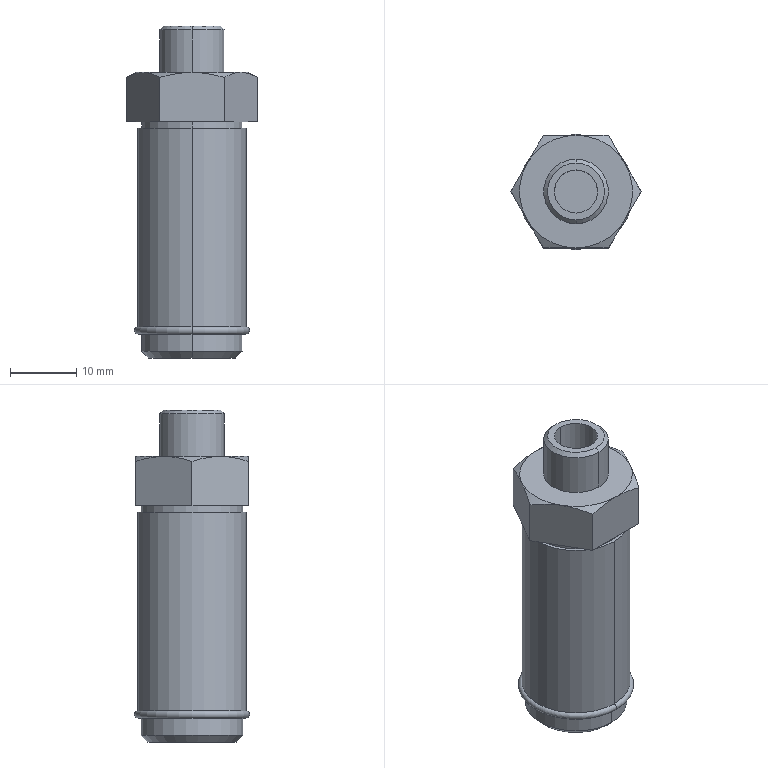Part | SolidWorks | features RefAxis 3, 3DProfileFeature 1, ICE 1, Revolution 1 | 1 solid | 40 faces | box 19.63 x 17.35 x 50 mm | volume 8637 mm3 | plane 14 | cylinder 12 | cone 12 | torus 2 | commonest cylinder face diameters 15.3 x4 6.485 x2 8.566 x2 9.728 x2 16.3 x2
STEP:
#1=CARTESIAN_POINT('',(0.,-4.864,39.4));
#2=VERTEX_POINT('',#1);
#3=CARTESIAN_POINT('',(0.,4.864,39.4));
#4=VERTEX_POINT('',#3);
#5=CARTESIAN_POINT('',(0.,0.,39.4));
#6=DIRECTION('',(0.,0.,1.));
#7=DIRECTION('',(0.,-1.,0.));
#8=AXIS2_PLACEMENT_3D('',#5,#6,#7);
#9=CIRCLE('',#8,4.864);
#10=EDGE_CURVE('',#2,#4,#9,.T.);
#11=ORIENTED_EDGE('',*,*,#10,.T.);
#12=CARTESIAN_POINT('',(0.,4.864,45.819));
#13=VERTEX_POINT('',#12);
#14=CARTESIAN_POINT('',(0.,4.864,-3.6));
#15=DIRECTION('',(0.,0.,1.));
#16=VECTOR('',#15,1000.);
#17=LINE('',#14,#16);
#18=EDGE_CURVE('',#4,#13,#17,.T.);
#19=ORIENTED_EDGE('',*,*,#18,.T.);
#20=CARTESIAN_POINT('',(0.,-4.864,45.819));
#21=VERTEX_POINT('',#20);
#22=CARTESIAN_POINT('',(0.,0.,45.819));
#23=DIRECTION('',(0.,0.,1.));
#24=DIRECTION('',(0.,-1.,0.));
#25=AXIS2_PLACEMENT_3D('',#22,#23,#24);
#26=CIRCLE('',#25,4.864);
#27=EDGE_CURVE('',#21,#13,#26,.T.);
#28=ORIENTED_EDGE('',*,*,#27,.F.);
#29=CARTESIAN_POINT('',(0.,-4.864,-3.6));
#30=DIRECTION('',(0.,0.,1.));
#31=VECTOR('',#30,1000.);
#32=LINE('',#29,#31);
#33=EDGE_CURVE('',#2,#21,#32,.T.);
#34=ORIENTED_EDGE('',*,*,#33,.F.);
#35=EDGE_LOOP('',(#11,#19,#28,#34));
#36=FACE_OUTER_BOUND('',#35,.T.);
#37=CARTESIAN_POINT('',(0.,0.,-3.6));
#38=DIRECTION('',(0.,0.,1.));
#39=DIRECTION('',(0.,-1.,0.));
#40=AXIS2_PLACEMENT_3D('',#37,#38,#39);
#41=CYLINDRICAL_SURFACE('',#40,4.864);
#42=ADVANCED_FACE('',(#36),#41,.T.);
#43=CARTESIAN_POINT('',(0.,-4.283,46.4));
#44=VERTEX_POINT('',#43);
#45=CARTESIAN_POINT('',(0.,4.283,46.4));
#46=VERTEX_POINT('',#45);
#47=CARTESIAN_POINT('',(0.,0.,46.4));
#48=DIRECTION('',(0.,0.,1.));
#49=DIRECTION('',(0.,-1.,0.));
#50=AXIS2_PLACEMENT_3D('',#47,#48,#49);
#51=CIRCLE('',#50,4.283);
#52=EDGE_CURVE('',#44,#46,#51,.T.);
#53=ORIENTED_EDGE('',*,*,#52,.F.);
#54=CARTESIAN_POINT('',(0.,-4.864,45.819));
#55=DIRECTION('',(0.,-0.7071,-0.7071));
#56=VECTOR('',#55,1000.);
#57=LINE('',#54,#56);
#58=EDGE_CURVE('',#44,#21,#57,.T.);
#59=ORIENTED_EDGE('',*,*,#58,.T.);
#60=ORIENTED_EDGE('',*,*,#27,.T.);
#61=CARTESIAN_POINT('',(0.,4.864,45.819));
#62=DIRECTION('',(0.,0.7071,-0.7071));
#63=VECTOR('',#62,1000.);
#64=LINE('',#61,#63);
#65=EDGE_CURVE('',#46,#13,#64,.T.);
#66=ORIENTED_EDGE('',*,*,#65,.F.);
#67=EDGE_LOOP('',(#53,#59,#60,#66));
#68=FACE_OUTER_BOUND('',#67,.T.);
#69=CARTESIAN_POINT('',(0.,0.,45.819));
#70=DIRECTION('',(0.,0.,-1.));
#71=DIRECTION('',(0.,1.,0.));
#72=AXIS2_PLACEMENT_3D('',#69,#70,#71);
#73=CONICAL_SURFACE('',#72,4.864,0.7854);
#74=ADVANCED_FACE('',(#68),#73,.T.);
#75=CARTESIAN_POINT('',(0.,3.243,26.4));
#76=VERTEX_POINT('',#75);
#77=CARTESIAN_POINT('',(0.,-3.243,26.4));
#78=VERTEX_POINT('',#77);
#79=CARTESIAN_POINT('',(0.,0.,26.4));
#80=DIRECTION('',(0.,0.,1.));
#81=DIRECTION('',(0.,-1.,0.));
#82=AXIS2_PLACEMENT_3D('',#79,#80,#81);
#83=CIRCLE('',#82,3.243);
#84=EDGE_CURVE('',#76,#78,#83,.T.);
#85=ORIENTED_EDGE('',*,*,#84,.F.);
#86=CARTESIAN_POINT('',(0.,3.243,46.4));
#87=VERTEX_POINT('',#86);
#88=CARTESIAN_POINT('',(0.,3.243,-3.6));
#89=DIRECTION('',(0.,0.,1.));
#90=VECTOR('',#89,1000.);
#91=LINE('',#88,#90);
#92=EDGE_CURVE('',#76,#87,#91,.T.);
#93=ORIENTED_EDGE('',*,*,#92,.T.);
#94=CARTESIAN_POINT('',(0.,-3.243,46.4));
#95=VERTEX_POINT('',#94);
#96=CARTESIAN_POINT('',(0.,0.,46.4));
#97=DIRECTION('',(0.,0.,1.));
#98=DIRECTION('',(0.,-1.,0.));
#99=AXIS2_PLACEMENT_3D('',#96,#97,#98);
#100=CIRCLE('',#99,3.243);
#101=EDGE_CURVE('',#87,#95,#100,.T.);
#102=ORIENTED_EDGE('',*,*,#101,.T.);
#103=CARTESIAN_POINT('',(0.,-3.243,-3.6));
#104=DIRECTION('',(0.,0.,1.));
#105=VECTOR('',#104,1000.);
#106=LINE('',#103,#105);
#107=EDGE_CURVE('',#78,#95,#106,.T.);
#108=ORIENTED_EDGE('',*,*,#107,.F.);
#109=EDGE_LOOP('',(#85,#93,#102,#108));
#110=FACE_OUTER_BOUND('',#109,.T.);
#111=CARTESIAN_POINT('',(0.,0.,-3.6));
#112=DIRECTION('',(0.,0.,1.));
#113=DIRECTION('',(0.,-1.,0.));
#114=AXIS2_PLACEMENT_3D('',#111,#112,#113);
#115=CYLINDRICAL_SURFACE('',#114,3.243);
#116=ADVANCED_FACE('',(#110),#115,.F.);
#117=CARTESIAN_POINT('',(0.,4.283,-3.019));
#118=VERTEX_POINT('',#117);
#119=CARTESIAN_POINT('',(0.,-4.283,-3.019));
#120=VERTEX_POINT('',#119);
#121=CARTESIAN_POINT('',(0.,0.,-3.019));
#122=DIRECTION('',(0.,0.,1.));
#123=DIRECTION('',(0.,-1.,0.));
#124=AXIS2_PLACEMENT_3D('',#121,#122,#123);
#125=CIRCLE('',#124,4.283);
#126=EDGE_CURVE('',#118,#120,#125,.T.);
#127=ORIENTED_EDGE('',*,*,#126,.F.);
#128=CARTESIAN_POINT('',(0.,4.283,2.9));
#129=VERTEX_POINT('',#128);
#130=CARTESIAN_POINT('',(0.,4.283,-3.6));
#131=DIRECTION('',(0.,0.,1.));
#132=VECTOR('',#131,1000.);
#133=LINE('',#130,#132);
#134=EDGE_CURVE('',#118,#129,#133,.T.);
#135=ORIENTED_EDGE('',*,*,#134,.T.);
#136=CARTESIAN_POINT('',(0.,-4.283,2.9));
#137=VERTEX_POINT('',#136);
#138=CARTESIAN_POINT('',(0.,0.,2.9));
#139=DIRECTION('',(0.,0.,1.));
#140=DIRECTION('',(0.,-1.,0.));
#141=AXIS2_PLACEMENT_3D('',#138,#139,#140);
#142=CIRCLE('',#141,4.283);
#143=EDGE_CURVE('',#129,#137,#142,.T.);
#144=ORIENTED_EDGE('',*,*,#143,.T.);
#145=CARTESIAN_POINT('',(0.,-4.283,-3.6));
#146=DIRECTION('',(0.,0.,1.));
#147=VECTOR('',#146,1000.);
#148=LINE('',#145,#147);
#149=EDGE_CURVE('',#120,#137,#148,.T.);
#150=ORIENTED_EDGE('',*,*,#149,.F.);
#151=EDGE_LOOP('',(#127,#135,#144,#150));
#152=FACE_OUTER_BOUND('',#151,.T.);
#153=CARTESIAN_POINT('',(0.,0.,-3.6));
#154=DIRECTION('',(0.,0.,1.));
#155=DIRECTION('',(0.,-1.,0.));
#156=AXIS2_PLACEMENT_3D('',#153,#154,#155);
#157=CYLINDRICAL_SURFACE('',#156,4.283);
#158=ADVANCED_FACE('',(#152),#157,.F.);
#159=ORIENTED_EDGE('',*,*,#126,.T.);
#160=CARTESIAN_POINT('',(0.,-4.864,-3.6));
#161=VERTEX_POINT('',#160);
#162=CARTESIAN_POINT('',(0.,-4.283,-3.019));
#163=DIRECTION('',(0.,-0.7071,-0.7071));
#164=VECTOR('',#163,1000.);
#165=LINE('',#162,#164);
#166=EDGE_CURVE('',#120,#161,#165,.T.);
#167=ORIENTED_EDGE('',*,*,#166,.T.);
#168=CARTESIAN_POINT('',(0.,4.864,-3.6));
#169=VERTEX_POINT('',#168);
#170=CARTESIAN_POINT('',(0.,0.,-3.6));
#171=DIRECTION('',(0.,0.,1.));
#172=DIRECTION('',(0.,-1.,0.));
#173=AXIS2_PLACEMENT_3D('',#170,#171,#172);
#174=CIRCLE('',#173,4.864);
#175=EDGE_CURVE('',#169,#161,#174,.T.);
#176=ORIENTED_EDGE('',*,*,#175,.F.);
#177=CARTESIAN_POINT('',(0.,4.283,-3.019));
#178=DIRECTION('',(0.,0.7071,-0.7071));
#179=VECTOR('',#178,1000.);
#180=LINE('',#177,#179);
#181=EDGE_CURVE('',#118,#169,#180,.T.);
#182=ORIENTED_EDGE('',*,*,#181,.F.);
#183=EDGE_LOOP('',(#159,#167,#176,#182));
#184=FACE_OUTER_BOUND('',#183,.T.);
#185=CARTESIAN_POINT('',(0.,0.,-3.019));
#186=DIRECTION('',(0.,0.,-1.));
#187=DIRECTION('',(0.,1.,0.));
#188=AXIS2_PLACEMENT_3D('',#185,#186,#187);
#189=CONICAL_SURFACE('',#188,4.283,0.7854);
#190=ADVANCED_FACE('',(#184),#189,.F.);
#191=CARTESIAN_POINT('',(0.,-6.65,-3.6));
#192=VERTEX_POINT('',#191);
#193=CARTESIAN_POINT('',(0.,6.65,-3.6));
#194=VERTEX_POINT('',#193);
#195=CARTESIAN_POINT('',(0.,0.,-3.6));
#196=DIRECTION('',(0.,0.,1.));
#197=DIRECTION('',(0.,-1.,0.));
#198=AXIS2_PLACEMENT_3D('',#195,#196,#197);
#199=CIRCLE('',#198,6.65);
#200=EDGE_CURVE('',#192,#194,#199,.T.);
#201=ORIENTED_EDGE('',*,*,#200,.T.);
#202=CARTESIAN_POINT('',(0.,7.65,-2.6));
#203=VERTEX_POINT('',#202);
#204=CARTESIAN_POINT('',(0.,6.65,-3.6));
#205=DIRECTION('',(0.,0.7071,0.7071));
#206=VECTOR('',#205,1000.);
#207=LINE('',#204,#206);
#208=EDGE_CURVE('',#194,#203,#207,.T.);
#209=ORIENTED_EDGE('',*,*,#208,.T.);
#210=CARTESIAN_POINT('',(0.,-7.65,-2.6));
#211=VERTEX_POINT('',#210);
#212=CARTESIAN_POINT('',(0.,0.,-2.6));
#213=DIRECTION('',(0.,0.,1.));
#214=DIRECTION('',(0.,-1.,0.));
#215=AXIS2_PLACEMENT_3D('',#212,#213,#214);
#216=CIRCLE('',#215,7.65);
#217=EDGE_CURVE('',#211,#203,#216,.T.);
#218=ORIENTED_EDGE('',*,*,#217,.F.);
#219=CARTESIAN_POINT('',(0.,-6.65,-3.6));
#220=DIRECTION('',(0.,-0.7071,0.7071));
#221=VECTOR('',#220,1000.);
#222=LINE('',#219,#221);
#223=EDGE_CURVE('',#192,#211,#222,.T.);
#224=ORIENTED_EDGE('',*,*,#223,.F.);
#225=EDGE_LOOP('',(#201,#209,#218,#224));
#226=FACE_OUTER_BOUND('',#225,.T.);
#227=CARTESIAN_POINT('',(0.,0.,-3.6));
#228=DIRECTION('',(0.,0.,1.));
#229=DIRECTION('',(0.,-1.,0.));
#230=AXIS2_PLACEMENT_3D('',#227,#228,#229);
#231=CONICAL_SURFACE('',#230,6.65,0.7854);
#232=ADVANCED_FACE('',(#226),#231,.T.);
#233=ORIENTED_EDGE('',*,*,#217,.T.);
#234=CARTESIAN_POINT('',(0.,7.65,0.));
#235=VERTEX_POINT('',#234);
#236=CARTESIAN_POINT('',(0.,7.65,-3.6));
#237=DIRECTION('',(0.,0.,1.));
#238=VECTOR('',#237,1000.);
#239=LINE('',#236,#238);
#240=EDGE_CURVE('',#203,#235,#239,.T.);
#241=ORIENTED_EDGE('',*,*,#240,.T.);
#242=CARTESIAN_POINT('',(0.,-7.65,0.));
#243=VERTEX_POINT('',#242);
#244=CARTESIAN_POINT('',(0.,0.,0.));
#245=DIRECTION('',(0.,0.,1.));
#246=DIRECTION('',(0.,-1.,0.));
#247=AXIS2_PLACEMENT_3D('',#244,#245,#246);
#248=CIRCLE('',#247,7.65);
#249=EDGE_CURVE('',#243,#235,#248,.T.);
#250=ORIENTED_EDGE('',*,*,#249,.F.);
#251=CARTESIAN_POINT('',(0.,-7.65,-3.6));
#252=DIRECTION('',(0.,0.,1.));
#253=VECTOR('',#252,1000.);
#254=LINE('',#251,#253);
#255=EDGE_CURVE('',#211,#243,#254,.T.);
#256=ORIENTED_EDGE('',*,*,#255,.F.);
#257=EDGE_LOOP('',(#233,#241,#250,#256));
#258=FACE_OUTER_BOUND('',#257,.T.);
#259=CARTESIAN_POINT('',(0.,0.,-3.6));
#260=DIRECTION('',(0.,0.,1.));
#261=DIRECTION('',(0.,-1.,0.));
#262=AXIS2_PLACEMENT_3D('',#259,#260,#261);
#263=CYLINDRICAL_SURFACE('',#262,7.65);
#264=ADVANCED_FACE('',(#258),#263,.T.);
#265=CARTESIAN_POINT('',(0.,-8.125,0.));
#266=VERTEX_POINT('',#265);
#267=CARTESIAN_POINT('',(0.,8.125,0.));
#268=VERTEX_POINT('',#267);
#269=CARTESIAN_POINT('',(0.,0.,0.));
#270=DIRECTION('',(0.,0.,1.));
#271=DIRECTION('',(0.,-1.,0.));
#272=AXIS2_PLACEMENT_3D('',#269,#270,#271);
#273=CIRCLE('',#272,8.125);
#274=EDGE_CURVE('',#266,#268,#273,.T.);
#275=ORIENTED_EDGE('',*,*,#274,.T.);
#276=CARTESIAN_POINT('',(0.,8.15,1.099));
#277=VERTEX_POINT('',#276);
#278=CARTESIAN_POINT('',(0.,8.125,0.55));
#279=DIRECTION('',(1.,0.,0.));
#280=DIRECTION('',(0.,1.,0.));
#281=AXIS2_PLACEMENT_3D('',#278,#279,#280);
#282=CIRCLE('',#281,0.55);
#283=EDGE_CURVE('',#268,#277,#282,.T.);
#284=ORIENTED_EDGE('',*,*,#283,.T.);
#285=CARTESIAN_POINT('',(0.,-8.15,1.099));
#286=VERTEX_POINT('',#285);
#287=CARTESIAN_POINT('',(0.,0.,1.099));
#288=DIRECTION('',(0.,0.,1.));
#289=DIRECTION('',(0.,-1.,0.));
#290=AXIS2_PLACEMENT_3D('',#287,#288,#289);
#291=CIRCLE('',#290,8.15);
#292=EDGE_CURVE('',#286,#277,#291,.T.);
#293=ORIENTED_EDGE('',*,*,#292,.F.);
#294=CARTESIAN_POINT('',(0.,-8.125,0.55));
#295=DIRECTION('',(-1.,0.,0.));
#296=DIRECTION('',(0.,0.,1.));
#297=AXIS2_PLACEMENT_3D('',#294,#295,#296);
#298=CIRCLE('',#297,0.55);
#299=EDGE_CURVE('',#266,#286,#298,.T.);
#300=ORIENTED_EDGE('',*,*,#299,.F.);
#301=EDGE_LOOP('',(#275,#284,#293,#300));
#302=FACE_OUTER_BOUND('',#301,.T.);
#303=CARTESIAN_POINT('',(0.,0.,0.55));
#304=DIRECTION('',(0.,0.,1.));
#305=DIRECTION('',(0.,-1.,0.));
#306=AXIS2_PLACEMENT_3D('',#303,#304,#305);
#307=TOROIDAL_SURFACE('',#306,8.125,0.55);
#308=ADVANCED_FACE('',(#302),#307,.T.);
#309=ORIENTED_EDGE('',*,*,#292,.T.);
#310=CARTESIAN_POINT('',(0.,8.15,31.));
#311=VERTEX_POINT('',#310);
#312=CARTESIAN_POINT('',(0.,8.15,-3.6));
#313=DIRECTION('',(0.,0.,1.));
#314=VECTOR('',#313,1000.);
#315=LINE('',#312,#314);
#316=EDGE_CURVE('',#277,#311,#315,.T.);
#317=ORIENTED_EDGE('',*,*,#316,.T.);
#318=CARTESIAN_POINT('',(0.,-8.15,31.));
#319=VERTEX_POINT('',#318);
#320=CARTESIAN_POINT('',(0.,0.,31.));
#321=DIRECTION('',(0.,0.,1.));
#322=DIRECTION('',(0.,-1.,0.));
#323=AXIS2_PLACEMENT_3D('',#320,#321,#322);
#324=CIRCLE('',#323,8.15);
#325=EDGE_CURVE('',#319,#311,#324,.T.);
#326=ORIENTED_EDGE('',*,*,#325,.F.);
#327=CARTESIAN_POINT('',(0.,-8.15,-3.6));
#328=DIRECTION('',(0.,0.,1.));
#329=VECTOR('',#328,1000.);
#330=LINE('',#327,#329);
#331=EDGE_CURVE('',#286,#319,#330,.T.);
#332=ORIENTED_EDGE('',*,*,#331,.F.);
#333=EDGE_LOOP('',(#309,#317,#326,#332));
#334=FACE_OUTER_BOUND('',#333,.T.);
#335=CARTESIAN_POINT('',(0.,0.,-3.6));
#336=DIRECTION('',(0.,0.,1.));
#337=DIRECTION('',(0.,-1.,0.));
#338=AXIS2_PLACEMENT_3D('',#335,#336,#337);
#339=CYLINDRICAL_SURFACE('',#338,8.15);
#340=ADVANCED_FACE('',(#334),#339,.T.);
#341=CARTESIAN_POINT('',(0.,-7.65,31.));
#342=VERTEX_POINT('',#341);
#343=CARTESIAN_POINT('',(0.,7.65,31.));
#344=VERTEX_POINT('',#343);
#345=CARTESIAN_POINT('',(0.,0.,31.));
#346=DIRECTION('',(0.,0.,1.));
#347=DIRECTION('',(0.,-1.,0.));
#348=AXIS2_PLACEMENT_3D('',#345,#346,#347);
#349=CIRCLE('',#348,7.65);
#350=EDGE_CURVE('',#342,#344,#349,.T.);
#351=ORIENTED_EDGE('',*,*,#350,.T.);
#352=CARTESIAN_POINT('',(0.,7.65,32.));
#353=VERTEX_POINT('',#352);
#354=CARTESIAN_POINT('',(0.,7.65,-3.6));
#355=DIRECTION('',(0.,0.,1.));
#356=VECTOR('',#355,1000.);
#357=LINE('',#354,#356);
#358=EDGE_CURVE('',#344,#353,#357,.T.);
#359=ORIENTED_EDGE('',*,*,#358,.T.);
#360=CARTESIAN_POINT('',(0.,-7.65,32.));
#361=VERTEX_POINT('',#360);
#362=CARTESIAN_POINT('',(0.,0.,32.));
#363=DIRECTION('',(0.,0.,1.));
#364=DIRECTION('',(0.,-1.,0.));
#365=AXIS2_PLACEMENT_3D('',#362,#363,#364);
#366=CIRCLE('',#365,7.65);
#367=EDGE_CURVE('',#361,#353,#366,.T.);
#368=ORIENTED_EDGE('',*,*,#367,.F.);
#369=CARTESIAN_POINT('',(0.,-7.65,-3.6));
#370=DIRECTION('',(0.,0.,1.));
#371=VECTOR('',#370,1000.);
#372=LINE('',#369,#371);
#373=EDGE_CURVE('',#342,#361,#372,.T.);
#374=ORIENTED_EDGE('',*,*,#373,.F.);
#375=EDGE_LOOP('',(#351,#359,#368,#374));
#376=FACE_OUTER_BOUND('',#375,.T.);
#377=CARTESIAN_POINT('',(0.,0.,-3.6));
#378=DIRECTION('',(0.,0.,1.));
#379=DIRECTION('',(0.,-1.,0.));
#380=AXIS2_PLACEMENT_3D('',#377,#378,#379);
#381=CYLINDRICAL_SURFACE('',#380,7.65);
#382=ADVANCED_FACE('',(#376),#381,.T.);
#383=ORIENTED_EDGE('',*,*,#367,.T.);
#384=CARTESIAN_POINT('',(0.,0.,32.));
#385=DIRECTION('',(0.,0.,1.));
#386=DIRECTION('',(0.,-1.,0.));
#387=AXIS2_PLACEMENT_3D('',#384,#385,#386);
#388=CIRCLE('',#387,7.65);
#389=EDGE_CURVE('',#353,#361,#388,.T.);
#390=ORIENTED_EDGE('',*,*,#389,.T.);
#391=EDGE_LOOP('',(#383,#390));
#392=FACE_BOUND('',#391,.T.);
#393=CARTESIAN_POINT('',(-9.815,0.,32.));
#394=VERTEX_POINT('',#393);
#395=CARTESIAN_POINT('',(-4.907,-8.5,32.));
#396=VERTEX_POINT('',#395);
#397=CARTESIAN_POINT('',(-9.815,0.,32.));
#398=DIRECTION('',(0.5,-0.866,0.));
#399=VECTOR('',#398,1000.);
#400=LINE('',#397,#399);
#401=EDGE_CURVE('',#394,#396,#400,.T.);
#402=ORIENTED_EDGE('',*,*,#401,.F.);
#403=CARTESIAN_POINT('',(-4.907,8.5,32.));
#404=VERTEX_POINT('',#403);
#405=CARTESIAN_POINT('',(-4.907,8.5,32.));
#406=DIRECTION('',(-0.5,-0.866,0.));
#407=VECTOR('',#406,1000.);
#408=LINE('',#405,#407);
#409=EDGE_CURVE('',#404,#394,#408,.T.);
#410=ORIENTED_EDGE('',*,*,#409,.F.);
#411=CARTESIAN_POINT('',(4.907,8.5,32.));
#412=VERTEX_POINT('',#411);
#413=CARTESIAN_POINT('',(4.907,8.5,32.));
#414=DIRECTION('',(-1.,0.,0.));
#415=VECTOR('',#414,1000.);
#416=LINE('',#413,#415);
#417=EDGE_CURVE('',#412,#404,#416,.T.);
#418=ORIENTED_EDGE('',*,*,#417,.F.);
#419=CARTESIAN_POINT('',(9.815,0.,32.));
#420=VERTEX_POINT('',#419);
#421=CARTESIAN_POINT('',(9.815,0.,32.));
#422=DIRECTION('',(-0.5,0.866,0.));
#423=VECTOR('',#422,1000.);
#424=LINE('',#421,#423);
#425=EDGE_CURVE('',#420,#412,#424,.T.);
#426=ORIENTED_EDGE('',*,*,#425,.F.);
#427=CARTESIAN_POINT('',(4.907,-8.5,32.));
#428=VERTEX_POINT('',#427);
#429=CARTESIAN_POINT('',(4.907,-8.5,32.));
#430=DIRECTION('',(0.5,0.866,0.));
#431=VECTOR('',#430,1000.);
#432=LINE('',#429,#431);
#433=EDGE_CURVE('',#428,#420,#432,.T.);
#434=ORIENTED_EDGE('',*,*,#433,.F.);
#435=CARTESIAN_POINT('',(-4.907,-8.5,32.));
#436=DIRECTION('',(1.,0.,0.));
#437=VECTOR('',#436,1000.);
#438=LINE('',#435,#437);
#439=EDGE_CURVE('',#396,#428,#438,.T.);
#440=ORIENTED_EDGE('',*,*,#439,.F.);
#441=EDGE_LOOP('',(#402,#410,#418,#426,#434,#440));
#442=FACE_OUTER_BOUND('',#441,.T.);
#443=CARTESIAN_POINT('',(0.,17.,32.));
#444=DIRECTION('',(0.,0.,1.));
#445=DIRECTION('',(0.,-1.,0.));
#446=AXIS2_PLACEMENT_3D('',#443,#444,#445);
#447=PLANE('',#446);
#448=ADVANCED_FACE('',(#392,#442),#447,.F.);
#449=ORIENTED_EDGE('',*,*,#358,.F.);
#450=CARTESIAN_POINT('',(0.,0.,31.));
#451=DIRECTION('',(0.,0.,1.));
#452=DIRECTION('',(0.,-1.,0.));
#453=AXIS2_PLACEMENT_3D('',#450,#451,#452);
#454=CIRCLE('',#453,7.65);
#455=EDGE_CURVE('',#344,#342,#454,.T.);
#456=ORIENTED_EDGE('',*,*,#455,.T.);
#457=ORIENTED_EDGE('',*,*,#373,.T.);
#458=ORIENTED_EDGE('',*,*,#389,.F.);
#459=EDGE_LOOP('',(#449,#456,#457,#458));
#460=FACE_OUTER_BOUND('',#459,.T.);
#461=CARTESIAN_POINT('',(0.,0.,-3.6));
#462=DIRECTION('',(0.,0.,1.));
#463=DIRECTION('',(0.,-1.,0.));
#464=AXIS2_PLACEMENT_3D('',#461,#462,#463);
#465=CYLINDRICAL_SURFACE('',#464,7.65);
#466=ADVANCED_FACE('',(#460),#465,.T.);
#467=ORIENTED_EDGE('',*,*,#350,.F.);
#468=ORIENTED_EDGE('',*,*,#455,.F.);
#469=EDGE_LOOP('',(#467,#468));
#470=FACE_BOUND('',#469,.T.);
#471=ORIENTED_EDGE('',*,*,#325,.T.);
#472=CARTESIAN_POINT('',(0.,0.,31.));
#473=DIRECTION('',(0.,0.,1.));
#474=DIRECTION('',(0.,-1.,0.));
#475=AXIS2_PLACEMENT_3D('',#472,#473,#474);
#476=CIRCLE('',#475,8.15);
#477=EDGE_CURVE('',#311,#319,#476,.T.);
#478=ORIENTED_EDGE('',*,*,#477,.T.);
#479=EDGE_LOOP('',(#471,#478));
#480=FACE_OUTER_BOUND('',#479,.T.);
#481=CARTESIAN_POINT('',(0.,7.65,31.));
#482=DIRECTION('',(0.,0.,-1.));
#483=DIRECTION('',(0.,1.,0.));
#484=AXIS2_PLACEMENT_3D('',#481,#482,#483);
#485=PLANE('',#484);
#486=ADVANCED_FACE('',(#470,#480),#485,.F.);
#487=ORIENTED_EDGE('',*,*,#316,.F.);
#488=CARTESIAN_POINT('',(0.,0.,1.099));
#489=DIRECTION('',(0.,0.,1.));
#490=DIRECTION('',(0.,-1.,0.));
#491=AXIS2_PLACEMENT_3D('',#488,#489,#490);
#492=CIRCLE('',#491,8.15);
#493=EDGE_CURVE('',#277,#286,#492,.T.);
#494=ORIENTED_EDGE('',*,*,#493,.T.);
#495=ORIENTED_EDGE('',*,*,#331,.T.);
#496=ORIENTED_EDGE('',*,*,#477,.F.);
#497=EDGE_LOOP('',(#487,#494,#495,#496));
#498=FACE_OUTER_BOUND('',#497,.T.);
#499=CARTESIAN_POINT('',(0.,0.,-3.6));
#500=DIRECTION('',(0.,0.,1.));
#501=DIRECTION('',(0.,-1.,0.));
#502=AXIS2_PLACEMENT_3D('',#499,#500,#501);
#503=CYLINDRICAL_SURFACE('',#502,8.15);
#504=ADVANCED_FACE('',(#498),#503,.T.);
#505=ORIENTED_EDGE('',*,*,#283,.F.);
#506=CARTESIAN_POINT('',(0.,0.,0.));
#507=DIRECTION('',(0.,0.,1.));
#508=DIRECTION('',(0.,-1.,0.));
#509=AXIS2_PLACEMENT_3D('',#506,#507,#508);
#510=CIRCLE('',#509,8.125);
#511=EDGE_CURVE('',#268,#266,#510,.T.);
#512=ORIENTED_EDGE('',*,*,#511,.T.);
#513=ORIENTED_EDGE('',*,*,#299,.T.);
#514=ORIENTED_EDGE('',*,*,#493,.F.);
#515=EDGE_LOOP('',(#505,#512,#513,#514));
#516=FACE_OUTER_BOUND('',#515,.T.);
#517=CARTESIAN_POINT('',(0.,0.,0.55));
#518=DIRECTION('',(0.,0.,1.));
#519=DIRECTION('',(0.,-1.,0.));
#520=AXIS2_PLACEMENT_3D('',#517,#518,#519);
#521=TOROIDAL_SURFACE('',#520,8.125,0.55);
#522=ADVANCED_FACE('',(#516),#521,.T.);
#523=ORIENTED_EDGE('',*,*,#274,.F.);
#524=ORIENTED_EDGE('',*,*,#511,.F.);
#525=EDGE_LOOP('',(#523,#524));
#526=FACE_OUTER_BOUND('',#525,.T.);
#527=ORIENTED_EDGE('',*,*,#249,.T.);
#528=CARTESIAN_POINT('',(0.,0.,0.));
#529=DIRECTION('',(0.,0.,1.));
#530=DIRECTION('',(0.,-1.,0.));
#531=AXIS2_PLACEMENT_3D('',#528,#529,#530);
#532=CIRCLE('',#531,7.65);
#533=EDGE_CURVE('',#235,#243,#532,.T.);
#534=ORIENTED_EDGE('',*,*,#533,.T.);
#535=EDGE_LOOP('',(#527,#534));
#536=FACE_BOUND('',#535,.T.);
#537=CARTESIAN_POINT('',(0.,8.125,0.));
#538=DIRECTION('',(0.,0.,1.));
#539=DIRECTION('',(0.,-1.,0.));
#540=AXIS2_PLACEMENT_3D('',#537,#538,#539);
#541=PLANE('',#540);
#542=ADVANCED_FACE('',(#526,#536),#541,.F.);
#543=ORIENTED_EDGE('',*,*,#240,.F.);
#544=CARTESIAN_POINT('',(0.,0.,-2.6));
#545=DIRECTION('',(0.,0.,1.));
#546=DIRECTION('',(0.,-1.,0.));
#547=AXIS2_PLACEMENT_3D('',#544,#545,#546);
#548=CIRCLE('',#547,7.65);
#549=EDGE_CURVE('',#203,#211,#548,.T.);
#550=ORIENTED_EDGE('',*,*,#549,.T.);
#551=ORIENTED_EDGE('',*,*,#255,.T.);
#552=ORIENTED_EDGE('',*,*,#533,.F.);
#553=EDGE_LOOP('',(#543,#550,#551,#552));
#554=FACE_OUTER_BOUND('',#553,.T.);
#555=CARTESIAN_POINT('',(0.,0.,-3.6));
#556=DIRECTION('',(0.,0.,1.));
#557=DIRECTION('',(0.,-1.,0.));
#558=AXIS2_PLACEMENT_3D('',#555,#556,#557);
#559=CYLINDRICAL_SURFACE('',#558,7.65);
#560=ADVANCED_FACE('',(#554),#559,.T.);
#561=ORIENTED_EDGE('',*,*,#208,.F.);
#562=CARTESIAN_POINT('',(0.,0.,-3.6));
#563=DIRECTION('',(0.,0.,1.));
#564=DIRECTION('',(0.,-1.,0.));
#565=AXIS2_PLACEMENT_3D('',#562,#563,#564);
#566=CIRCLE('',#565,6.65);
#567=EDGE_CURVE('',#194,#192,#566,.T.);
#568=ORIENTED_EDGE('',*,*,#567,.T.);
#569=ORIENTED_EDGE('',*,*,#223,.T.);
#570=ORIENTED_EDGE('',*,*,#549,.F.);
#571=EDGE_LOOP('',(#561,#568,#569,#570));
#572=FACE_OUTER_BOUND('',#571,.T.);
#573=CARTESIAN_POINT('',(0.,0.,-3.6));
#574=DIRECTION('',(0.,0.,1.));
#575=DIRECTION('',(0.,-1.,0.));
#576=AXIS2_PLACEMENT_3D('',#573,#574,#575);
#577=CONICAL_SURFACE('',#576,6.65,0.7854);
#578=ADVANCED_FACE('',(#572),#577,.T.);
#579=ORIENTED_EDGE('',*,*,#200,.F.);
#580=ORIENTED_EDGE('',*,*,#567,.F.);
#581=EDGE_LOOP('',(#579,#580));
#582=FACE_OUTER_BOUND('',#581,.T.);
#583=ORIENTED_EDGE('',*,*,#175,.T.);
#584=CARTESIAN_POINT('',(0.,0.,-3.6));
#585=DIRECTION('',(0.,0.,1.));
#586=DIRECTION('',(0.,-1.,0.));
#587=AXIS2_PLACEMENT_3D('',#584,#585,#586);
#588=CIRCLE('',#587,4.864);
#589=EDGE_CURVE('',#161,#169,#588,.T.);
#590=ORIENTED_EDGE('',*,*,#589,.T.);
#591=EDGE_LOOP('',(#583,#590));
#592=FACE_BOUND('',#591,.T.);
#593=CARTESIAN_POINT('',(0.,6.65,-3.6));
#594=DIRECTION('',(0.,0.,1.));
#595=DIRECTION('',(0.,-1.,0.));
#596=AXIS2_PLACEMENT_3D('',#593,#594,#595);
#597=PLANE('',#596);
#598=ADVANCED_FACE('',(#582,#592),#597,.F.);
#599=ORIENTED_EDGE('',*,*,#166,.F.);
#600=CARTESIAN_POINT('',(0.,0.,-3.019));
#601=DIRECTION('',(0.,0.,1.));
#602=DIRECTION('',(0.,-1.,0.));
#603=AXIS2_PLACEMENT_3D('',#600,#601,#602);
#604=CIRCLE('',#603,4.283);
#605=EDGE_CURVE('',#120,#118,#604,.T.);
#606=ORIENTED_EDGE('',*,*,#605,.T.);
#607=ORIENTED_EDGE('',*,*,#181,.T.);
#608=ORIENTED_EDGE('',*,*,#589,.F.);
#609=EDGE_LOOP('',(#599,#606,#607,#608));
#610=FACE_OUTER_BOUND('',#609,.T.);
#611=CARTESIAN_POINT('',(0.,0.,-3.019));
#612=DIRECTION('',(0.,0.,-1.));
#613=DIRECTION('',(0.,1.,0.));
#614=AXIS2_PLACEMENT_3D('',#611,#612,#613);
#615=CONICAL_SURFACE('',#614,4.283,0.7854);
#616=ADVANCED_FACE('',(#610),#615,.F.);
#617=ORIENTED_EDGE('',*,*,#134,.F.);
#618=ORIENTED_EDGE('',*,*,#605,.F.);
#619=ORIENTED_EDGE('',*,*,#149,.T.);
#620=CARTESIAN_POINT('',(0.,0.,2.9));
#621=DIRECTION('',(0.,0.,1.));
#622=DIRECTION('',(0.,-1.,0.));
#623=AXIS2_PLACEMENT_3D('',#620,#621,#622);
#624=CIRCLE('',#623,4.283);
#625=EDGE_CURVE('',#137,#129,#624,.T.);
#626=ORIENTED_EDGE('',*,*,#625,.T.);
#627=EDGE_LOOP('',(#617,#618,#619,#626));
#628=FACE_OUTER_BOUND('',#627,.T.);
#629=CARTESIAN_POINT('',(0.,0.,-3.6));
#630=DIRECTION('',(0.,0.,1.));
#631=DIRECTION('',(0.,-1.,0.));
#632=AXIS2_PLACEMENT_3D('',#629,#630,#631);
#633=CYLINDRICAL_SURFACE('',#632,4.283);
#634=ADVANCED_FACE('',(#628),#633,.F.);
#635=ORIENTED_EDGE('',*,*,#625,.F.);
#636=ORIENTED_EDGE('',*,*,#143,.F.);
#637=EDGE_LOOP('',(#635,#636));
#638=FACE_OUTER_BOUND('',#637,.T.);
#639=CARTESIAN_POINT('',(0.,4.283,2.9));
#640=DIRECTION('',(0.,0.,1.));
#641=DIRECTION('',(0.,-1.,0.));
#642=AXIS2_PLACEMENT_3D('',#639,#640,#641);
#643=PLANE('',#642);
#644=ADVANCED_FACE('',(#638),#643,.F.);
#645=CARTESIAN_POINT('',(-4.907,-8.5,38.641));
#646=VERTEX_POINT('',#645);
#647=CARTESIAN_POINT('',(-7.361,-4.25,39.4));
#648=VERTEX_POINT('',#647);
#649=CARTESIAN_POINT('',(-4.907,-8.5,38.641));
#650=CARTESIAN_POINT('',(-5.309,-7.805,38.873));
#651=CARTESIAN_POINT('',(-5.713,-7.104,39.063));
#652=CARTESIAN_POINT('',(-6.53,-5.689,39.328));
#653=CARTESIAN_POINT('',(-6.943,-4.974,39.4));
#654=CARTESIAN_POINT('',(-7.361,-4.25,39.4));
#655=B_SPLINE_CURVE_WITH_KNOTS('',3,(#649,#650,#651,#652,#653,#654),.UNSPECIFIED.,.F.,.F.,(4,2,4),(0.000000238,0.002483,0.004966),.UNSPECIFIED.);
#656=EDGE_CURVE('',#646,#648,#655,.T.);
#657=ORIENTED_EDGE('',*,*,#656,.T.);
#658=CARTESIAN_POINT('',(-9.815,0.,38.641));
#659=VERTEX_POINT('',#658);
#660=CARTESIAN_POINT('',(-7.361,-4.25,39.4));
#661=CARTESIAN_POINT('',(-7.569,-3.889,39.4));
#662=CARTESIAN_POINT('',(-7.779,-3.527,39.382));
#663=CARTESIAN_POINT('',(-8.192,-2.81,39.313));
#664=CARTESIAN_POINT('',(-8.398,-2.454,39.261));
#665=CARTESIAN_POINT('',(-9.011,-1.393,39.063));
#666=CARTESIAN_POINT('',(-9.415,-0.6935,38.872));
#667=CARTESIAN_POINT('',(-9.815,0.,38.641));
#668=B_SPLINE_CURVE_WITH_KNOTS('',3,(#660,#661,#662,#663,#664,#665,#666,#667),.UNSPECIFIED.,.F.,.F.,(4,2,2,4),(0.004966,0.006203,0.007439,0.009913),.UNSPECIFIED.);
#669=EDGE_CURVE('',#648,#659,#668,.T.);
#670=ORIENTED_EDGE('',*,*,#669,.T.);
#671=CARTESIAN_POINT('',(-9.815,0.,32.));
#672=DIRECTION('',(0.,0.,1.));
#673=VECTOR('',#672,1000.);
#674=LINE('',#671,#673);
#675=EDGE_CURVE('',#394,#659,#674,.T.);
#676=ORIENTED_EDGE('',*,*,#675,.F.);
#677=ORIENTED_EDGE('',*,*,#401,.T.);
#678=CARTESIAN_POINT('',(-4.907,-8.5,32.));
#679=DIRECTION('',(0.,0.,1.));
#680=VECTOR('',#679,1000.);
#681=LINE('',#678,#680);
#682=EDGE_CURVE('',#396,#646,#681,.T.);
#683=ORIENTED_EDGE('',*,*,#682,.T.);
#684=EDGE_LOOP('',(#657,#670,#676,#677,#683));
#685=FACE_OUTER_BOUND('',#684,.T.);
#686=CARTESIAN_POINT('',(-9.815,0.,32.));
#687=DIRECTION('',(-0.866,-0.5,0.));
#688=DIRECTION('',(0.5,-0.866,0.));
#689=AXIS2_PLACEMENT_3D('',#686,#687,#688);
#690=PLANE('',#689);
#691=ADVANCED_FACE('',(#685),#690,.T.);
#692=CARTESIAN_POINT('',(-7.361,4.25,39.4));
#693=VERTEX_POINT('',#692);
#694=CARTESIAN_POINT('',(-9.815,0.,38.641));
#695=CARTESIAN_POINT('',(-9.414,0.6952,38.873));
#696=CARTESIAN_POINT('',(-9.009,1.396,39.063));
#697=CARTESIAN_POINT('',(-8.192,2.811,39.328));
#698=CARTESIAN_POINT('',(-7.779,3.526,39.4));
#699=CARTESIAN_POINT('',(-7.361,4.25,39.4));
#700=B_SPLINE_CURVE_WITH_KNOTS('',3,(#694,#695,#696,#697,#698,#699),.UNSPECIFIED.,.F.,.F.,(4,2,4),(0.000000238,0.002483,0.004966),.UNSPECIFIED.);
#701=EDGE_CURVE('',#659,#693,#700,.T.);
#702=ORIENTED_EDGE('',*,*,#701,.T.);
#703=CARTESIAN_POINT('',(-4.907,8.5,38.641));
#704=VERTEX_POINT('',#703);
#705=CARTESIAN_POINT('',(-7.361,4.25,39.4));
#706=CARTESIAN_POINT('',(-7.153,4.611,39.4));
#707=CARTESIAN_POINT('',(-6.944,4.973,39.382));
#708=CARTESIAN_POINT('',(-6.53,5.69,39.313));
#709=CARTESIAN_POINT('',(-6.324,6.046,39.261));
#710=CARTESIAN_POINT('',(-5.712,7.107,39.063));
#711=CARTESIAN_POINT('',(-5.308,7.806,38.872));
#712=CARTESIAN_POINT('',(-4.907,8.5,38.641));
#713=B_SPLINE_CURVE_WITH_KNOTS('',3,(#705,#706,#707,#708,#709,#710,#711,#712),.UNSPECIFIED.,.F.,.F.,(4,2,2,4),(0.004966,0.006203,0.007439,0.009913),.UNSPECIFIED.);
#714=EDGE_CURVE('',#693,#704,#713,.T.);
#715=ORIENTED_EDGE('',*,*,#714,.T.);
#716=CARTESIAN_POINT('',(-4.907,8.5,32.));
#717=DIRECTION('',(0.,0.,1.));
#718=VECTOR('',#717,1000.);
#719=LINE('',#716,#718);
#720=EDGE_CURVE('',#404,#704,#719,.T.);
#721=ORIENTED_EDGE('',*,*,#720,.F.);
#722=ORIENTED_EDGE('',*,*,#409,.T.);
#723=ORIENTED_EDGE('',*,*,#675,.T.);
#724=EDGE_LOOP('',(#702,#715,#721,#722,#723));
#725=FACE_OUTER_BOUND('',#724,.T.);
#726=CARTESIAN_POINT('',(-4.907,8.5,32.));
#727=DIRECTION('',(-0.866,0.5,0.));
#728=DIRECTION('',(-0.5,-0.866,0.));
#729=AXIS2_PLACEMENT_3D('',#726,#727,#728);
#730=PLANE('',#729);
#731=ADVANCED_FACE('',(#725),#730,.T.);
#732=CARTESIAN_POINT('',(0.,8.5,39.4));
#733=VERTEX_POINT('',#732);
#734=CARTESIAN_POINT('',(-4.907,8.5,38.641));
#735=CARTESIAN_POINT('',(-4.109,8.5,38.871));
#736=CARTESIAN_POINT('',(-3.291,8.5,39.065));
#737=CARTESIAN_POINT('',(-1.654,8.5,39.329));
#738=CARTESIAN_POINT('',(-0.8301,8.5,39.4));
#739=CARTESIAN_POINT('',(0.,8.5,39.4));
#740=B_SPLINE_CURVE_WITH_KNOTS('',3,(#734,#735,#736,#737,#738,#739),.UNSPECIFIED.,.F.,.F.,(4,2,4),(0.009018,0.0115,0.01399),.UNSPECIFIED.);
#741=EDGE_CURVE('',#704,#733,#740,.T.);
#742=ORIENTED_EDGE('',*,*,#741,.T.);
#743=CARTESIAN_POINT('',(4.907,8.5,38.641));
#744=VERTEX_POINT('',#743);
#745=CARTESIAN_POINT('',(0.,8.5,39.4));
#746=CARTESIAN_POINT('',(0.4153,8.5,39.4));
#747=CARTESIAN_POINT('',(0.8327,8.5,39.382));
#748=CARTESIAN_POINT('',(1.668,8.5,39.312));
#749=CARTESIAN_POINT('',(2.082,8.5,39.26));
#750=CARTESIAN_POINT('',(3.31,8.5,39.061));
#751=CARTESIAN_POINT('',(4.114,8.5,38.87));
#752=CARTESIAN_POINT('',(4.907,8.5,38.641));
#753=B_SPLINE_CURVE_WITH_KNOTS('',3,(#745,#746,#747,#748,#749,#750,#751,#752),.UNSPECIFIED.,.F.,.F.,(4,2,2,4),(0.01399,0.01523,0.01647,0.01896),.UNSPECIFIED.);
#754=EDGE_CURVE('',#733,#744,#753,.T.);
#755=ORIENTED_EDGE('',*,*,#754,.T.);
#756=CARTESIAN_POINT('',(4.907,8.5,32.));
#757=DIRECTION('',(0.,0.,1.));
#758=VECTOR('',#757,1000.);
#759=LINE('',#756,#758);
#760=EDGE_CURVE('',#412,#744,#759,.T.);
#761=ORIENTED_EDGE('',*,*,#760,.F.);
#762=ORIENTED_EDGE('',*,*,#417,.T.);
#763=ORIENTED_EDGE('',*,*,#720,.T.);
#764=EDGE_LOOP('',(#742,#755,#761,#762,#763));
#765=FACE_OUTER_BOUND('',#764,.T.);
#766=CARTESIAN_POINT('',(4.907,8.5,32.));
#767=DIRECTION('',(0.,1.,0.));
#768=DIRECTION('',(0.,0.,1.));
#769=AXIS2_PLACEMENT_3D('',#766,#767,#768);
#770=PLANE('',#769);
#771=ADVANCED_FACE('',(#765),#770,.T.);
#772=CARTESIAN_POINT('',(7.361,4.25,39.4));
#773=VERTEX_POINT('',#772);
#774=CARTESIAN_POINT('',(4.907,8.5,38.641));
#775=CARTESIAN_POINT('',(5.309,7.805,38.873));
#776=CARTESIAN_POINT('',(5.713,7.104,39.063));
#777=CARTESIAN_POINT('',(6.53,5.689,39.328));
#778=CARTESIAN_POINT('',(6.943,4.974,39.4));
#779=CARTESIAN_POINT('',(7.361,4.25,39.4));
#780=B_SPLINE_CURVE_WITH_KNOTS('',3,(#774,#775,#776,#777,#778,#779),.UNSPECIFIED.,.F.,.F.,(4,2,4),(0.000000238,0.002483,0.004966),.UNSPECIFIED.);
#781=EDGE_CURVE('',#744,#773,#780,.T.);
#782=ORIENTED_EDGE('',*,*,#781,.T.);
#783=CARTESIAN_POINT('',(9.815,0.,38.641));
#784=VERTEX_POINT('',#783);
#785=CARTESIAN_POINT('',(7.361,4.25,39.4));
#786=CARTESIAN_POINT('',(7.569,3.889,39.4));
#787=CARTESIAN_POINT('',(7.779,3.527,39.382));
#788=CARTESIAN_POINT('',(8.192,2.81,39.313));
#789=CARTESIAN_POINT('',(8.398,2.454,39.261));
#790=CARTESIAN_POINT('',(9.011,1.393,39.063));
#791=CARTESIAN_POINT('',(9.415,0.6935,38.872));
#792=CARTESIAN_POINT('',(9.815,0.,38.641));
#793=B_SPLINE_CURVE_WITH_KNOTS('',3,(#785,#786,#787,#788,#789,#790,#791,#792),.UNSPECIFIED.,.F.,.F.,(4,2,2,4),(0.004966,0.006203,0.007439,0.009913),.UNSPECIFIED.);
#794=EDGE_CURVE('',#773,#784,#793,.T.);
#795=ORIENTED_EDGE('',*,*,#794,.T.);
#796=CARTESIAN_POINT('',(9.815,0.,32.));
#797=DIRECTION('',(0.,0.,1.));
#798=VECTOR('',#797,1000.);
#799=LINE('',#796,#798);
#800=EDGE_CURVE('',#420,#784,#799,.T.);
#801=ORIENTED_EDGE('',*,*,#800,.F.);
#802=ORIENTED_EDGE('',*,*,#425,.T.);
#803=ORIENTED_EDGE('',*,*,#760,.T.);
#804=EDGE_LOOP('',(#782,#795,#801,#802,#803));
#805=FACE_OUTER_BOUND('',#804,.T.);
#806=CARTESIAN_POINT('',(9.815,0.,32.));
#807=DIRECTION('',(0.866,0.5,0.));
#808=DIRECTION('',(-0.5,0.866,0.));
#809=AXIS2_PLACEMENT_3D('',#806,#807,#808);
#810=PLANE('',#809);
#811=ADVANCED_FACE('',(#805),#810,.T.);
#812=CARTESIAN_POINT('',(7.361,-4.25,39.4));
#813=VERTEX_POINT('',#812);
#814=CARTESIAN_POINT('',(9.815,0.,38.641));
#815=CARTESIAN_POINT('',(9.414,-0.6952,38.873));
#816=CARTESIAN_POINT('',(9.009,-1.396,39.063));
#817=CARTESIAN_POINT('',(8.192,-2.811,39.328));
#818=CARTESIAN_POINT('',(7.779,-3.526,39.4));
#819=CARTESIAN_POINT('',(7.361,-4.25,39.4));
#820=B_SPLINE_CURVE_WITH_KNOTS('',3,(#814,#815,#816,#817,#818,#819),.UNSPECIFIED.,.F.,.F.,(4,2,4),(0.000000238,0.002483,0.004966),.UNSPECIFIED.);
#821=EDGE_CURVE('',#784,#813,#820,.T.);
#822=ORIENTED_EDGE('',*,*,#821,.T.);
#823=CARTESIAN_POINT('',(4.907,-8.5,38.641));
#824=VERTEX_POINT('',#823);
#825=CARTESIAN_POINT('',(7.361,-4.25,39.4));
#826=CARTESIAN_POINT('',(7.153,-4.611,39.4));
#827=CARTESIAN_POINT('',(6.944,-4.973,39.382));
#828=CARTESIAN_POINT('',(6.53,-5.69,39.313));
#829=CARTESIAN_POINT('',(6.324,-6.046,39.261));
#830=CARTESIAN_POINT('',(5.712,-7.107,39.063));
#831=CARTESIAN_POINT('',(5.308,-7.806,38.872));
#832=CARTESIAN_POINT('',(4.907,-8.5,38.641));
#833=B_SPLINE_CURVE_WITH_KNOTS('',3,(#825,#826,#827,#828,#829,#830,#831,#832),.UNSPECIFIED.,.F.,.F.,(4,2,2,4),(0.004966,0.006203,0.007439,0.009913),.UNSPECIFIED.);
#834=EDGE_CURVE('',#813,#824,#833,.T.);
#835=ORIENTED_EDGE('',*,*,#834,.T.);
#836=CARTESIAN_POINT('',(4.907,-8.5,32.));
#837=DIRECTION('',(0.,0.,1.));
#838=VECTOR('',#837,1000.);
#839=LINE('',#836,#838);
#840=EDGE_CURVE('',#428,#824,#839,.T.);
#841=ORIENTED_EDGE('',*,*,#840,.F.);
#842=ORIENTED_EDGE('',*,*,#433,.T.);
#843=ORIENTED_EDGE('',*,*,#800,.T.);
#844=EDGE_LOOP('',(#822,#835,#841,#842,#843));
#845=FACE_OUTER_BOUND('',#844,.T.);
#846=CARTESIAN_POINT('',(4.907,-8.5,32.));
#847=DIRECTION('',(0.866,-0.5,0.));
#848=DIRECTION('',(0.5,0.866,0.));
#849=AXIS2_PLACEMENT_3D('',#846,#847,#848);
#850=PLANE('',#849);
#851=ADVANCED_FACE('',(#845),#850,.T.);
#852=CARTESIAN_POINT('',(0.,-8.5,39.4));
#853=VERTEX_POINT('',#852);
#854=CARTESIAN_POINT('',(4.907,-8.5,38.641));
#855=CARTESIAN_POINT('',(4.114,-8.5,38.87));
#856=CARTESIAN_POINT('',(3.31,-8.5,39.061));
#857=CARTESIAN_POINT('',(2.082,-8.5,39.26));
#858=CARTESIAN_POINT('',(1.668,-8.5,39.312));
#859=CARTESIAN_POINT('',(0.8327,-8.5,39.382));
#860=CARTESIAN_POINT('',(0.4153,-8.5,39.4));
#861=CARTESIAN_POINT('',(0.,-8.5,39.4));
#862=B_SPLINE_CURVE_WITH_KNOTS('',3,(#854,#855,#856,#857,#858,#859,#860,#861),.UNSPECIFIED.,.F.,.F.,(4,2,2,4),(0.02522,0.0277,0.02895,0.03019),.UNSPECIFIED.);
#863=EDGE_CURVE('',#824,#853,#862,.T.);
#864=ORIENTED_EDGE('',*,*,#863,.T.);
#865=CARTESIAN_POINT('',(0.,-8.5,39.4));
#866=CARTESIAN_POINT('',(-0.8301,-8.5,39.4));
#867=CARTESIAN_POINT('',(-1.654,-8.5,39.329));
#868=CARTESIAN_POINT('',(-3.291,-8.5,39.065));
#869=CARTESIAN_POINT('',(-4.109,-8.5,38.871));
#870=CARTESIAN_POINT('',(-4.907,-8.5,38.641));
#871=B_SPLINE_CURVE_WITH_KNOTS('',3,(#865,#866,#867,#868,#869,#870),.UNSPECIFIED.,.F.,.F.,(4,2,4),(0.03019,0.03267,0.03516),.UNSPECIFIED.);
#872=EDGE_CURVE('',#853,#646,#871,.T.);
#873=ORIENTED_EDGE('',*,*,#872,.T.);
#874=ORIENTED_EDGE('',*,*,#682,.F.);
#875=ORIENTED_EDGE('',*,*,#439,.T.);
#876=ORIENTED_EDGE('',*,*,#840,.T.);
#877=EDGE_LOOP('',(#864,#873,#874,#875,#876));
#878=FACE_OUTER_BOUND('',#877,.T.);
#879=CARTESIAN_POINT('',(-4.907,-8.5,32.));
#880=DIRECTION('',(0.,-1.,0.));
#881=DIRECTION('',(0.,0.,-1.));
#882=AXIS2_PLACEMENT_3D('',#879,#880,#881);
#883=PLANE('',#882);
#884=ADVANCED_FACE('',(#878),#883,.T.);
#885=CARTESIAN_POINT('',(0.,0.,26.4));
#886=DIRECTION('',(0.,0.,1.));
#887=DIRECTION('',(0.,-1.,0.));
#888=AXIS2_PLACEMENT_3D('',#885,#886,#887);
#889=CIRCLE('',#888,3.243);
#890=EDGE_CURVE('',#78,#76,#889,.T.);
#891=ORIENTED_EDGE('',*,*,#890,.T.);
#892=ORIENTED_EDGE('',*,*,#84,.T.);
#893=EDGE_LOOP('',(#891,#892));
#894=FACE_OUTER_BOUND('',#893,.T.);
#895=CARTESIAN_POINT('',(0.,0.,26.4));
#896=DIRECTION('',(0.,0.,-1.));
#897=DIRECTION('',(0.,1.,0.));
#898=AXIS2_PLACEMENT_3D('',#895,#896,#897);
#899=PLANE('',#898);
#900=ADVANCED_FACE('',(#894),#899,.F.);
#901=ORIENTED_EDGE('',*,*,#92,.F.);
#902=ORIENTED_EDGE('',*,*,#890,.F.);
#903=ORIENTED_EDGE('',*,*,#107,.T.);
#904=CARTESIAN_POINT('',(0.,0.,46.4));
#905=DIRECTION('',(0.,0.,1.));
#906=DIRECTION('',(0.,-1.,0.));
#907=AXIS2_PLACEMENT_3D('',#904,#905,#906);
#908=CIRCLE('',#907,3.243);
#909=EDGE_CURVE('',#95,#87,#908,.T.);
#910=ORIENTED_EDGE('',*,*,#909,.T.);
#911=EDGE_LOOP('',(#901,#902,#903,#910));
#912=FACE_OUTER_BOUND('',#911,.T.);
#913=CARTESIAN_POINT('',(0.,0.,-3.6));
#914=DIRECTION('',(0.,0.,1.));
#915=DIRECTION('',(0.,-1.,0.));
#916=AXIS2_PLACEMENT_3D('',#913,#914,#915);
#917=CYLINDRICAL_SURFACE('',#916,3.243);
#918=ADVANCED_FACE('',(#912),#917,.F.);
#919=ORIENTED_EDGE('',*,*,#909,.F.);
#920=ORIENTED_EDGE('',*,*,#101,.F.);
#921=EDGE_LOOP('',(#919,#920));
#922=FACE_BOUND('',#921,.T.);
#923=CARTESIAN_POINT('',(0.,0.,46.4));
#924=DIRECTION('',(0.,0.,1.));
#925=DIRECTION('',(0.,-1.,0.));
#926=AXIS2_PLACEMENT_3D('',#923,#924,#925);
#927=CIRCLE('',#926,4.283);
#928=EDGE_CURVE('',#46,#44,#927,.T.);
#929=ORIENTED_EDGE('',*,*,#928,.T.);
#930=ORIENTED_EDGE('',*,*,#52,.T.);
#931=EDGE_LOOP('',(#929,#930));
#932=FACE_OUTER_BOUND('',#931,.T.);
#933=CARTESIAN_POINT('',(0.,3.243,46.4));
#934=DIRECTION('',(0.,0.,-1.));
#935=DIRECTION('',(0.,1.,0.));
#936=AXIS2_PLACEMENT_3D('',#933,#934,#935);
#937=PLANE('',#936);
#938=ADVANCED_FACE('',(#922,#932),#937,.F.);
#939=ORIENTED_EDGE('',*,*,#58,.F.);
#940=ORIENTED_EDGE('',*,*,#928,.F.);
#941=ORIENTED_EDGE('',*,*,#65,.T.);
#942=CARTESIAN_POINT('',(0.,0.,45.819));
#943=DIRECTION('',(0.,0.,1.));
#944=DIRECTION('',(0.,-1.,0.));
#945=AXIS2_PLACEMENT_3D('',#942,#943,#944);
#946=CIRCLE('',#945,4.864);
#947=EDGE_CURVE('',#13,#21,#946,.T.);
#948=ORIENTED_EDGE('',*,*,#947,.T.);
#949=EDGE_LOOP('',(#939,#940,#941,#948));
#950=FACE_OUTER_BOUND('',#949,.T.);
#951=CARTESIAN_POINT('',(0.,0.,45.819));
#952=DIRECTION('',(0.,0.,-1.));
#953=DIRECTION('',(0.,1.,0.));
#954=AXIS2_PLACEMENT_3D('',#951,#952,#953);
#955=CONICAL_SURFACE('',#954,4.864,0.7854);
#956=ADVANCED_FACE('',(#950),#955,.T.);
#957=ORIENTED_EDGE('',*,*,#18,.F.);
#958=CARTESIAN_POINT('',(0.,0.,39.4));
#959=DIRECTION('',(0.,0.,1.));
#960=DIRECTION('',(0.,-1.,0.));
#961=AXIS2_PLACEMENT_3D('',#958,#959,#960);
#962=CIRCLE('',#961,4.864);
#963=EDGE_CURVE('',#4,#2,#962,.T.);
#964=ORIENTED_EDGE('',*,*,#963,.T.);
#965=ORIENTED_EDGE('',*,*,#33,.T.);
#966=ORIENTED_EDGE('',*,*,#947,.F.);
#967=EDGE_LOOP('',(#957,#964,#965,#966));
#968=FACE_OUTER_BOUND('',#967,.T.);
#969=CARTESIAN_POINT('',(0.,0.,-3.6));
#970=DIRECTION('',(0.,0.,1.));
#971=DIRECTION('',(0.,-1.,0.));
#972=AXIS2_PLACEMENT_3D('',#969,#970,#971);
#973=CYLINDRICAL_SURFACE('',#972,4.864);
#974=ADVANCED_FACE('',(#968),#973,.T.);
#975=ORIENTED_EDGE('',*,*,#669,.F.);
#976=CARTESIAN_POINT('',(0.,0.,39.4));
#977=DIRECTION('',(0.,0.,1.));
#978=DIRECTION('',(0.,-1.,0.));
#979=AXIS2_PLACEMENT_3D('',#976,#977,#978);
#980=CIRCLE('',#979,8.5);
#981=EDGE_CURVE('',#693,#648,#980,.T.);
#982=ORIENTED_EDGE('',*,*,#981,.F.);
#983=ORIENTED_EDGE('',*,*,#701,.F.);
#984=EDGE_LOOP('',(#975,#982,#983));
#985=FACE_OUTER_BOUND('',#984,.T.);
#986=CARTESIAN_POINT('',(0.,0.,34.493));
#987=DIRECTION('',(0.,0.,-1.));
#988=DIRECTION('',(0.,1.,0.));
#989=AXIS2_PLACEMENT_3D('',#986,#987,#988);
#990=CONICAL_SURFACE('',#989,17.,1.047);
#991=ADVANCED_FACE('',(#985),#990,.T.);
#992=ORIENTED_EDGE('',*,*,#714,.F.);
#993=CARTESIAN_POINT('',(0.,0.,39.4));
#994=DIRECTION('',(0.,0.,1.));
#995=DIRECTION('',(0.,-1.,0.));
#996=AXIS2_PLACEMENT_3D('',#993,#994,#995);
#997=CIRCLE('',#996,8.5);
#998=EDGE_CURVE('',#733,#693,#997,.T.);
#999=ORIENTED_EDGE('',*,*,#998,.F.);
#1000=ORIENTED_EDGE('',*,*,#741,.F.);
#1001=EDGE_LOOP('',(#992,#999,#1000));
#1002=FACE_OUTER_BOUND('',#1001,.T.);
#1003=CARTESIAN_POINT('',(0.,0.,34.493));
#1004=DIRECTION('',(0.,0.,-1.));
#1005=DIRECTION('',(0.,1.,0.));
#1006=AXIS2_PLACEMENT_3D('',#1003,#1004,#1005);
#1007=CONICAL_SURFACE('',#1006,17.,1.047);
#1008=ADVANCED_FACE('',(#1002),#1007,.T.);
#1009=ORIENTED_EDGE('',*,*,#754,.F.);
#1010=CARTESIAN_POINT('',(0.,0.,39.4));
#1011=DIRECTION('',(0.,0.,1.));
#1012=DIRECTION('',(0.,-1.,0.));
#1013=AXIS2_PLACEMENT_3D('',#1010,#1011,#1012);
#1014=CIRCLE('',#1013,8.5);
#1015=EDGE_CURVE('',#773,#733,#1014,.T.);
#1016=ORIENTED_EDGE('',*,*,#1015,.F.);
#1017=ORIENTED_EDGE('',*,*,#781,.F.);
#1018=EDGE_LOOP('',(#1009,#1016,#1017));
#1019=FACE_OUTER_BOUND('',#1018,.T.);
#1020=CARTESIAN_POINT('',(0.,0.,34.493));
#1021=DIRECTION('',(0.,0.,-1.));
#1022=DIRECTION('',(0.,1.,0.));
#1023=AXIS2_PLACEMENT_3D('',#1020,#1021,#1022);
#1024=CONICAL_SURFACE('',#1023,17.,1.047);
#1025=ADVANCED_FACE('',(#1019),#1024,.T.);
#1026=ORIENTED_EDGE('',*,*,#794,.F.);
#1027=CARTESIAN_POINT('',(0.,0.,39.4));
#1028=DIRECTION('',(0.,0.,1.));
#1029=DIRECTION('',(0.,-1.,0.));
#1030=AXIS2_PLACEMENT_3D('',#1027,#1028,#1029);
#1031=CIRCLE('',#1030,8.5);
#1032=EDGE_CURVE('',#813,#773,#1031,.T.);
#1033=ORIENTED_EDGE('',*,*,#1032,.F.);
#1034=ORIENTED_EDGE('',*,*,#821,.F.);
#1035=EDGE_LOOP('',(#1026,#1033,#1034));
#1036=FACE_OUTER_BOUND('',#1035,.T.);
#1037=CARTESIAN_POINT('',(0.,0.,34.493));
#1038=DIRECTION('',(0.,0.,-1.));
#1039=DIRECTION('',(0.,1.,0.));
#1040=AXIS2_PLACEMENT_3D('',#1037,#1038,#1039);
#1041=CONICAL_SURFACE('',#1040,17.,1.047);
#1042=ADVANCED_FACE('',(#1036),#1041,.T.);
#1043=ORIENTED_EDGE('',*,*,#834,.F.);
#1044=CARTESIAN_POINT('',(0.,0.,39.4));
#1045=DIRECTION('',(0.,0.,1.));
#1046=DIRECTION('',(0.,-1.,0.));
#1047=AXIS2_PLACEMENT_3D('',#1044,#1045,#1046);
#1048=CIRCLE('',#1047,8.5);
#1049=EDGE_CURVE('',#853,#813,#1048,.T.);
#1050=ORIENTED_EDGE('',*,*,#1049,.F.);
#1051=ORIENTED_EDGE('',*,*,#863,.F.);
#1052=EDGE_LOOP('',(#1043,#1050,#1051));
#1053=FACE_OUTER_BOUND('',#1052,.T.);
#1054=CARTESIAN_POINT('',(0.,0.,34.493));
#1055=DIRECTION('',(0.,0.,-1.));
#1056=DIRECTION('',(0.,1.,0.));
#1057=AXIS2_PLACEMENT_3D('',#1054,#1055,#1056);
#1058=CONICAL_SURFACE('',#1057,17.,1.047);
#1059=ADVANCED_FACE('',(#1053),#1058,.T.);
#1060=ORIENTED_EDGE('',*,*,#10,.F.);
#1061=ORIENTED_EDGE('',*,*,#963,.F.);
#1062=EDGE_LOOP('',(#1060,#1061));
#1063=FACE_BOUND('',#1062,.T.);
#1064=ORIENTED_EDGE('',*,*,#1049,.T.);
#1065=ORIENTED_EDGE('',*,*,#1032,.T.);
#1066=ORIENTED_EDGE('',*,*,#1015,.T.);
#1067=ORIENTED_EDGE('',*,*,#998,.T.);
#1068=ORIENTED_EDGE('',*,*,#981,.T.);
#1069=CARTESIAN_POINT('',(0.,0.,39.4));
#1070=DIRECTION('',(0.,0.,1.));
#1071=DIRECTION('',(0.,-1.,0.));
#1072=AXIS2_PLACEMENT_3D('',#1069,#1070,#1071);
#1073=CIRCLE('',#1072,8.5);
#1074=EDGE_CURVE('',#648,#853,#1073,.T.);
#1075=ORIENTED_EDGE('',*,*,#1074,.T.);
#1076=EDGE_LOOP('',(#1064,#1065,#1066,#1067,#1068,#1075));
#1077=FACE_OUTER_BOUND('',#1076,.T.);
#1078=CARTESIAN_POINT('',(0.,4.864,39.4));
#1079=DIRECTION('',(0.,0.,-1.));
#1080=DIRECTION('',(0.,1.,0.));
#1081=AXIS2_PLACEMENT_3D('',#1078,#1079,#1080);
#1082=PLANE('',#1081);
#1083=ADVANCED_FACE('',(#1063,#1077),#1082,.F.);
#1084=ORIENTED_EDGE('',*,*,#656,.F.);
#1085=ORIENTED_EDGE('',*,*,#872,.F.);
#1086=ORIENTED_EDGE('',*,*,#1074,.F.);
#1087=EDGE_LOOP('',(#1084,#1085,#1086));
#1088=FACE_OUTER_BOUND('',#1087,.T.);
#1089=CARTESIAN_POINT('',(0.,0.,34.493));
#1090=DIRECTION('',(0.,0.,-1.));
#1091=DIRECTION('',(0.,1.,0.));
#1092=AXIS2_PLACEMENT_3D('',#1089,#1090,#1091);
#1093=CONICAL_SURFACE('',#1092,17.,1.047);
#1094=ADVANCED_FACE('',(#1088),#1093,.T.);
#1095=CLOSED_SHELL('',(#42,#74,#116,#158,#190,#232,#264,#308,#340,#382,#448,#466,#486,#504,#522,#542,#560,#578,#598,#616,#634,#644,#691,#731,#771,#811,#851,#884,#900,#918,#938,#956,#974,#991,#1008,#1025,#1042,#1059,#1083,#1094));
#1096=MANIFOLD_SOLID_BREP('',#1095);
#1097=CARTESIAN_POINT('',(0.,0.,0.));
#1098=DIRECTION('',(0.,0.,1.));
#1099=DIRECTION('',(1.,0.,0.));
#1100=AXIS2_PLACEMENT_3D('',#1097,#1098,#1099);
#1101=(LENGTH_UNIT()NAMED_UNIT(*)SI_UNIT(.MILLI.,.METRE.));
#1102=UNCERTAINTY_MEASURE_WITH_UNIT(LENGTH_MEASURE(0.00001),#1101,'','');
#1103=(NAMED_UNIT(*)PLANE_ANGLE_UNIT()SI_UNIT($,.RADIAN.));
#1104=(NAMED_UNIT(*)SI_UNIT($,.STERADIAN.)SOLID_ANGLE_UNIT());
#1105=(GEOMETRIC_REPRESENTATION_CONTEXT(3)GLOBAL_UNCERTAINTY_ASSIGNED_CONTEXT((#1102))GLOBAL_UNIT_ASSIGNED_CONTEXT((#1101,#1103,#1104))REPRESENTATION_CONTEXT('',''));
#1106=ADVANCED_BREP_SHAPE_REPRESENTATION('',(#1096,#1100),#1105);